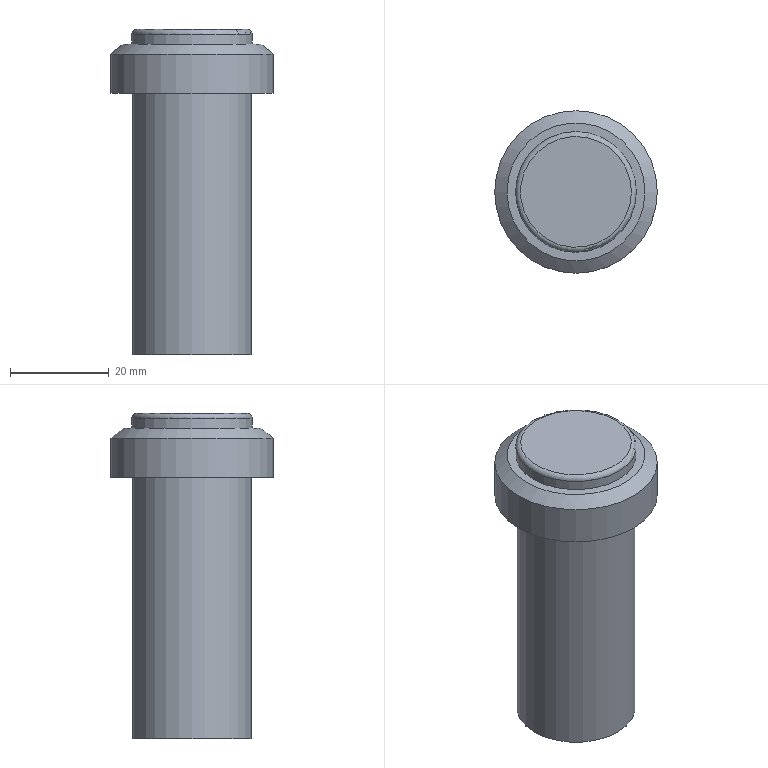Part | NX | 1 solid | 9 faces | box 33 x 33 x 66 mm | volume 33682 mm3 | plane 4 | cylinder 3 | cone 1 | torus 1 | commonest cylinder face diameters 24 x1 24.5 x1 33 x1
STEP:
#1=CARTESIAN_POINT('',(14.,0.,63.));
#2=VERTEX_POINT('',#1);
#3=CARTESIAN_POINT('',(0.,0.,63.));
#4=DIRECTION('',(0.,0.,1.));
#5=DIRECTION('',(1.,0.,0.));
#6=AXIS2_PLACEMENT_3D('',#3,#4,#5);
#7=CIRCLE('',#6,14.);
#8=EDGE_CURVE('',#2,#2,#7,.T.);
#9=ORIENTED_EDGE('',*,*,#8,.T.);
#10=EDGE_LOOP('',(#9));
#11=FACE_BOUND('',#10,.T.);
#12=CARTESIAN_POINT('',(12.25,0.,63.));
#13=VERTEX_POINT('',#12);
#14=CARTESIAN_POINT('',(0.,0.,63.));
#15=DIRECTION('',(0.,0.,1.));
#16=DIRECTION('',(1.,0.,0.));
#17=AXIS2_PLACEMENT_3D('',#14,#15,#16);
#18=CIRCLE('',#17,12.25);
#19=EDGE_CURVE('',#13,#13,#18,.T.);
#20=ORIENTED_EDGE('',*,*,#19,.F.);
#21=EDGE_LOOP('',(#20));
#22=FACE_BOUND('',#21,.T.);
#23=CARTESIAN_POINT('',(0.,0.,63.));
#24=DIRECTION('',(0.,0.,1.));
#25=DIRECTION('',(1.,0.,0.));
#26=AXIS2_PLACEMENT_3D('',#23,#24,#25);
#27=PLANE('',#26);
#28=ADVANCED_FACE('',(#11,#22),#27,.T.);
#29=CARTESIAN_POINT('',(12.,0.,53.));
#30=VERTEX_POINT('',#29);
#31=CARTESIAN_POINT('',(0.,0.,53.));
#32=DIRECTION('',(0.,0.,1.));
#33=DIRECTION('',(1.,0.,0.));
#34=AXIS2_PLACEMENT_3D('',#31,#32,#33);
#35=CIRCLE('',#34,12.);
#36=EDGE_CURVE('',#30,#30,#35,.T.);
#37=ORIENTED_EDGE('',*,*,#36,.F.);
#38=EDGE_LOOP('',(#37));
#39=FACE_BOUND('',#38,.T.);
#40=CARTESIAN_POINT('',(12.,0.,0.));
#41=VERTEX_POINT('',#40);
#42=CARTESIAN_POINT('',(0.,0.,0.));
#43=DIRECTION('',(0.,0.,1.));
#44=DIRECTION('',(1.,0.,0.));
#45=AXIS2_PLACEMENT_3D('',#42,#43,#44);
#46=CIRCLE('',#45,12.);
#47=EDGE_CURVE('',#41,#41,#46,.T.);
#48=ORIENTED_EDGE('',*,*,#47,.T.);
#49=EDGE_LOOP('',(#48));
#50=FACE_BOUND('',#49,.T.);
#51=CARTESIAN_POINT('',(0.,0.,53.));
#52=DIRECTION('',(0.,0.,-1.));
#53=DIRECTION('',(-1.,0.,0.));
#54=AXIS2_PLACEMENT_3D('',#51,#52,#53);
#55=CYLINDRICAL_SURFACE('',#54,12.);
#56=ADVANCED_FACE('',(#39,#50),#55,.T.);
#57=ORIENTED_EDGE('',*,*,#47,.F.);
#58=EDGE_LOOP('',(#57));
#59=FACE_BOUND('',#58,.T.);
#60=CARTESIAN_POINT('',(0.,0.,0.));
#61=DIRECTION('',(0.,0.,1.));
#62=DIRECTION('',(1.,0.,0.));
#63=AXIS2_PLACEMENT_3D('',#60,#61,#62);
#64=PLANE('',#63);
#65=ADVANCED_FACE('',(#59),#64,.F.);
#66=CARTESIAN_POINT('',(16.5,0.,53.));
#67=VERTEX_POINT('',#66);
#68=CARTESIAN_POINT('',(0.,0.,53.));
#69=DIRECTION('',(0.,0.,1.));
#70=DIRECTION('',(1.,0.,0.));
#71=AXIS2_PLACEMENT_3D('',#68,#69,#70);
#72=CIRCLE('',#71,16.5);
#73=EDGE_CURVE('',#67,#67,#72,.T.);
#74=ORIENTED_EDGE('',*,*,#73,.F.);
#75=EDGE_LOOP('',(#74));
#76=FACE_BOUND('',#75,.T.);
#77=ORIENTED_EDGE('',*,*,#36,.T.);
#78=EDGE_LOOP('',(#77));
#79=FACE_BOUND('',#78,.T.);
#80=CARTESIAN_POINT('',(0.,0.,53.));
#81=DIRECTION('',(0.,0.,1.));
#82=DIRECTION('',(1.,0.,0.));
#83=AXIS2_PLACEMENT_3D('',#80,#81,#82);
#84=PLANE('',#83);
#85=ADVANCED_FACE('',(#76,#79),#84,.F.);
#86=CARTESIAN_POINT('',(16.5,0.,61.));
#87=VERTEX_POINT('',#86);
#88=CARTESIAN_POINT('',(0.,0.,61.));
#89=DIRECTION('',(0.,0.,1.));
#90=DIRECTION('',(1.,0.,0.));
#91=AXIS2_PLACEMENT_3D('',#88,#89,#90);
#92=CIRCLE('',#91,16.5);
#93=EDGE_CURVE('',#87,#87,#92,.F.);
#94=ORIENTED_EDGE('',*,*,#93,.T.);
#95=EDGE_LOOP('',(#94));
#96=FACE_BOUND('',#95,.T.);
#97=ORIENTED_EDGE('',*,*,#73,.T.);
#98=EDGE_LOOP('',(#97));
#99=FACE_BOUND('',#98,.T.);
#100=CARTESIAN_POINT('',(0.,0.,63.));
#101=DIRECTION('',(0.,0.,-1.));
#102=DIRECTION('',(-1.,0.,0.));
#103=AXIS2_PLACEMENT_3D('',#100,#101,#102);
#104=CYLINDRICAL_SURFACE('',#103,16.5);
#105=ADVANCED_FACE('',(#96,#99),#104,.T.);
#106=ORIENTED_EDGE('',*,*,#93,.F.);
#107=EDGE_LOOP('',(#106));
#108=FACE_BOUND('',#107,.T.);
#109=ORIENTED_EDGE('',*,*,#8,.F.);
#110=EDGE_LOOP('',(#109));
#111=FACE_BOUND('',#110,.T.);
#112=CARTESIAN_POINT('',(0.,0.,63.));
#113=DIRECTION('',(0.,0.,-1.));
#114=DIRECTION('',(-1.,0.,0.));
#115=AXIS2_PLACEMENT_3D('',#112,#113,#114);
#116=CONICAL_SURFACE('',#115,14.,0.8961);
#117=ADVANCED_FACE('',(#108,#111),#116,.T.);
#118=CARTESIAN_POINT('',(12.25,0.,65.));
#119=VERTEX_POINT('',#118);
#120=CARTESIAN_POINT('',(0.,0.,65.));
#121=DIRECTION('',(0.,0.,1.));
#122=DIRECTION('',(1.,0.,0.));
#123=AXIS2_PLACEMENT_3D('',#120,#121,#122);
#124=CIRCLE('',#123,12.25);
#125=EDGE_CURVE('',#119,#119,#124,.F.);
#126=ORIENTED_EDGE('',*,*,#125,.T.);
#127=EDGE_LOOP('',(#126));
#128=FACE_BOUND('',#127,.T.);
#129=ORIENTED_EDGE('',*,*,#19,.T.);
#130=EDGE_LOOP('',(#129));
#131=FACE_BOUND('',#130,.T.);
#132=CARTESIAN_POINT('',(0.,0.,66.));
#133=DIRECTION('',(0.,0.,-1.));
#134=DIRECTION('',(-1.,0.,0.));
#135=AXIS2_PLACEMENT_3D('',#132,#133,#134);
#136=CYLINDRICAL_SURFACE('',#135,12.25);
#137=ADVANCED_FACE('',(#128,#131),#136,.T.);
#138=CARTESIAN_POINT('',(11.25,0.,66.));
#139=VERTEX_POINT('',#138);
#140=CARTESIAN_POINT('',(0.,0.,66.));
#141=DIRECTION('',(0.,0.,1.));
#142=DIRECTION('',(1.,0.,0.));
#143=AXIS2_PLACEMENT_3D('',#140,#141,#142);
#144=CIRCLE('',#143,11.25);
#145=EDGE_CURVE('',#139,#139,#144,.T.);
#146=ORIENTED_EDGE('',*,*,#145,.T.);
#147=EDGE_LOOP('',(#146));
#148=FACE_BOUND('',#147,.T.);
#149=CARTESIAN_POINT('',(0.,0.,66.));
#150=DIRECTION('',(0.,0.,1.));
#151=DIRECTION('',(1.,0.,0.));
#152=AXIS2_PLACEMENT_3D('',#149,#150,#151);
#153=PLANE('',#152);
#154=ADVANCED_FACE('',(#148),#153,.T.);
#155=ORIENTED_EDGE('',*,*,#125,.F.);
#156=EDGE_LOOP('',(#155));
#157=FACE_BOUND('',#156,.T.);
#158=ORIENTED_EDGE('',*,*,#145,.F.);
#159=EDGE_LOOP('',(#158));
#160=FACE_BOUND('',#159,.T.);
#161=CARTESIAN_POINT('',(0.,0.,65.));
#162=DIRECTION('',(0.,0.,1.));
#163=DIRECTION('',(1.,0.,0.));
#164=AXIS2_PLACEMENT_3D('',#161,#162,#163);
#165=TOROIDAL_SURFACE('',#164,11.25,1.);
#166=ADVANCED_FACE('',(#157,#160),#165,.T.);
#167=CLOSED_SHELL('',(#28,#56,#65,#85,#105,#117,#137,#154,#166));
#168=MANIFOLD_SOLID_BREP('',#167);
#169=(LENGTH_UNIT()NAMED_UNIT(*)SI_UNIT(.MILLI.,.METRE.));
#170=UNCERTAINTY_MEASURE_WITH_UNIT(LENGTH_MEASURE(0.00001),#169,'','');
#171=(NAMED_UNIT(*)PLANE_ANGLE_UNIT()SI_UNIT($,.RADIAN.));
#172=(NAMED_UNIT(*)SI_UNIT($,.STERADIAN.)SOLID_ANGLE_UNIT());
#173=(GEOMETRIC_REPRESENTATION_CONTEXT(3)GLOBAL_UNCERTAINTY_ASSIGNED_CONTEXT((#170))GLOBAL_UNIT_ASSIGNED_CONTEXT((#169,#171,#172))REPRESENTATION_CONTEXT('',''));
#174=ADVANCED_BREP_SHAPE_REPRESENTATION('',(#168),#173);